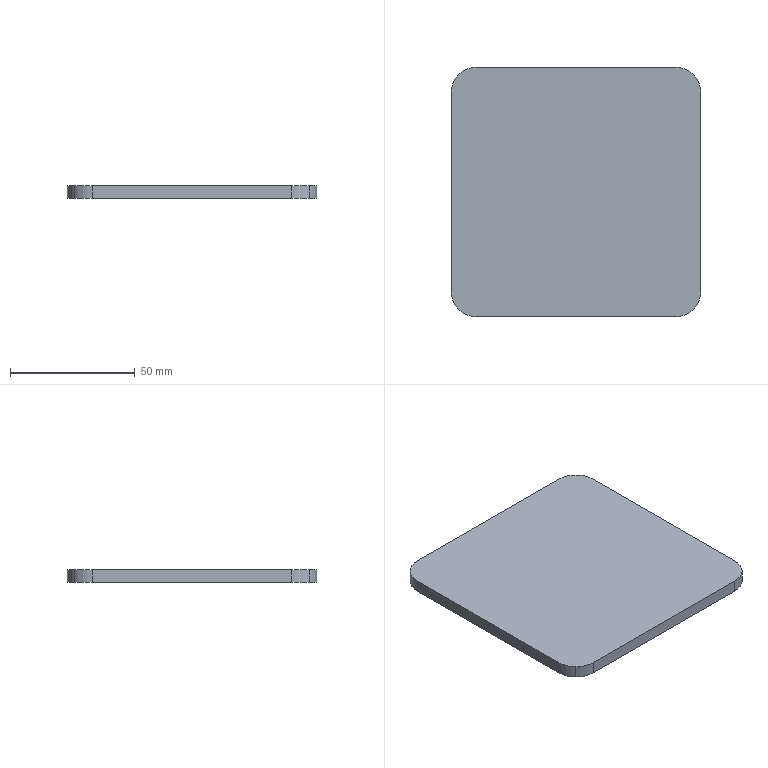Part | STEP file | DCV-000-024 | 1 solid | 14 faces | box 100 x 100 x 5 mm | volume 49571 mm3 | cylinder 8 | plane 6 | commonest cylinder face diameters 20 x8
STEP:
#1=CARTESIAN_POINT('',(0.,0.,0.));
#2=DIRECTION('',(0.,0.,1.));
#3=DIRECTION('',(1.,0.,0.));
#4=AXIS2_PLACEMENT_3D('',#1,#2,#3);
#5=CARTESIAN_POINT('',(40.,-50.,0.));
#6=VERTEX_POINT('',#5);
#7=CARTESIAN_POINT('',(47.071,-47.071,0.));
#8=VERTEX_POINT('',#7);
#9=CARTESIAN_POINT('',(40.,-40.,0.));
#10=DIRECTION('',(0.,0.,1.));
#11=DIRECTION('',(0.7071,-0.7071,0.));
#12=AXIS2_PLACEMENT_3D('',#9,#10,#11);
#13=CIRCLE('',#12,10.);
#14=CARTESIAN_POINT('',(40.,-40.,0.));
#15=DIRECTION('',(0.,0.,1.));
#16=DIRECTION('',(0.7071,-0.7071,0.));
#17=AXIS2_PLACEMENT_3D('',#14,#15,#16);
#18=CYLINDRICAL_SURFACE('',#17,10.);
#19=CARTESIAN_POINT('',(0.,0.));
#20=DIRECTION('',(1.,0.));
#21=VECTOR('',#20,1.);
#22=LINE('',#19,#21);
#23=(GEOMETRIC_REPRESENTATION_CONTEXT(2)PARAMETRIC_REPRESENTATION_CONTEXT()REPRESENTATION_CONTEXT('',''));
#24=DEFINITIONAL_REPRESENTATION('',(#22),#23);
#25=PCURVE('',#18,#24);
#26=CARTESIAN_POINT('',(0.,0.,0.));
#27=DIRECTION('',(0.,0.,1.));
#28=DIRECTION('',(1.,0.,0.));
#29=AXIS2_PLACEMENT_3D('',#26,#27,#28);
#30=PLANE('',#29);
#31=CARTESIAN_POINT('',(40.,-40.));
#32=DIRECTION('',(0.7071,-0.7071));
#33=AXIS2_PLACEMENT_2D('',#31,#32);
#34=CIRCLE('',#33,10.);
#35=(GEOMETRIC_REPRESENTATION_CONTEXT(2)PARAMETRIC_REPRESENTATION_CONTEXT()REPRESENTATION_CONTEXT('',''));
#36=DEFINITIONAL_REPRESENTATION('',(#34),#35);
#37=PCURVE('',#30,#36);
#38=SURFACE_CURVE('',#13,(#25,#37),.PCURVE_S1.);
#39=EDGE_CURVE('',#6,#8,#38,.T.);
#40=ORIENTED_EDGE('',*,*,#39,.T.);
#41=CARTESIAN_POINT('',(47.071,-47.071,5.));
#42=VERTEX_POINT('',#41);
#43=CARTESIAN_POINT('',(47.071,-47.071,0.));
#44=DIRECTION('',(0.,0.,1.));
#45=VECTOR('',#44,1.);
#46=LINE('',#43,#45);
#47=CARTESIAN_POINT('',(6.283,0.));
#48=DIRECTION('',(0.,1.));
#49=VECTOR('',#48,1.);
#50=LINE('',#47,#49);
#51=(GEOMETRIC_REPRESENTATION_CONTEXT(2)PARAMETRIC_REPRESENTATION_CONTEXT()REPRESENTATION_CONTEXT('',''));
#52=DEFINITIONAL_REPRESENTATION('',(#50),#51);
#53=PCURVE('',#18,#52);
#54=CARTESIAN_POINT('',(40.,-40.,0.));
#55=DIRECTION('',(0.,0.,1.));
#56=DIRECTION('',(0.7071,-0.7071,0.));
#57=AXIS2_PLACEMENT_3D('',#54,#55,#56);
#58=CYLINDRICAL_SURFACE('',#57,10.);
#59=CARTESIAN_POINT('',(0.,0.));
#60=DIRECTION('',(0.,1.));
#61=VECTOR('',#60,1.);
#62=LINE('',#59,#61);
#63=(GEOMETRIC_REPRESENTATION_CONTEXT(2)PARAMETRIC_REPRESENTATION_CONTEXT()REPRESENTATION_CONTEXT('',''));
#64=DEFINITIONAL_REPRESENTATION('',(#62),#63);
#65=PCURVE('',#58,#64);
#66=SURFACE_CURVE('',#46,(#53,#65),.PCURVE_S1.);
#67=EDGE_CURVE('',#8,#42,#66,.T.);
#68=ORIENTED_EDGE('',*,*,#67,.T.);
#69=CARTESIAN_POINT('',(40.,-50.,5.));
#70=VERTEX_POINT('',#69);
#71=CARTESIAN_POINT('',(40.,-40.,5.));
#72=DIRECTION('',(0.,0.,-1.));
#73=DIRECTION('',(0.7071,-0.7071,0.));
#74=AXIS2_PLACEMENT_3D('',#71,#72,#73);
#75=CIRCLE('',#74,10.);
#76=CARTESIAN_POINT('',(6.283,5.));
#77=DIRECTION('',(-1.,0.));
#78=VECTOR('',#77,1.);
#79=LINE('',#76,#78);
#80=(GEOMETRIC_REPRESENTATION_CONTEXT(2)PARAMETRIC_REPRESENTATION_CONTEXT()REPRESENTATION_CONTEXT('',''));
#81=DEFINITIONAL_REPRESENTATION('',(#79),#80);
#82=PCURVE('',#18,#81);
#83=CARTESIAN_POINT('',(0.,0.,5.));
#84=DIRECTION('',(0.,0.,1.));
#85=DIRECTION('',(1.,0.,0.));
#86=AXIS2_PLACEMENT_3D('',#83,#84,#85);
#87=PLANE('',#86);
#88=CARTESIAN_POINT('',(47.071,-47.071));
#89=CARTESIAN_POINT('',(34.824,-59.319));
#90=CARTESIAN_POINT('',(30.341,-42.588));
#91=CARTESIAN_POINT('',(25.858,-25.858));
#92=CARTESIAN_POINT('',(42.588,-30.341));
#93=CARTESIAN_POINT('',(59.319,-34.824));
#94=CARTESIAN_POINT('',(47.071,-47.071));
#95=(BOUNDED_CURVE()B_SPLINE_CURVE(2,(#88,#89,#90,#91,#92,#93,#94),.UNSPECIFIED.,.T.,.F.)B_SPLINE_CURVE_WITH_KNOTS((1,2,2,2,2,1),(-2.094,0.,2.094,4.189,6.283,8.378),.UNSPECIFIED.)CURVE()GEOMETRIC_REPRESENTATION_ITEM()RATIONAL_B_SPLINE_CURVE((1.,0.5,1.,0.5,1.,0.5,1.))REPRESENTATION_ITEM(''));
#96=(GEOMETRIC_REPRESENTATION_CONTEXT(2)PARAMETRIC_REPRESENTATION_CONTEXT()REPRESENTATION_CONTEXT('',''));
#97=DEFINITIONAL_REPRESENTATION('',(#95),#96);
#98=PCURVE('',#87,#97);
#99=SURFACE_CURVE('',#75,(#82,#98),.PCURVE_S1.);
#100=EDGE_CURVE('',#42,#70,#99,.T.);
#101=ORIENTED_EDGE('',*,*,#100,.T.);
#102=CARTESIAN_POINT('',(40.,-50.,0.));
#103=DIRECTION('',(0.,0.,-1.));
#104=VECTOR('',#103,1.);
#105=LINE('',#102,#104);
#106=CARTESIAN_POINT('',(5.498,0.));
#107=DIRECTION('',(0.,-1.));
#108=VECTOR('',#107,1.);
#109=LINE('',#106,#108);
#110=(GEOMETRIC_REPRESENTATION_CONTEXT(2)PARAMETRIC_REPRESENTATION_CONTEXT()REPRESENTATION_CONTEXT('',''));
#111=DEFINITIONAL_REPRESENTATION('',(#109),#110);
#112=PCURVE('',#18,#111);
#113=CARTESIAN_POINT('',(-50.,-50.,0.));
#114=DIRECTION('',(0.,-1.,0.));
#115=DIRECTION('',(0.,0.,-1.));
#116=AXIS2_PLACEMENT_3D('',#113,#114,#115);
#117=PLANE('',#116);
#118=CARTESIAN_POINT('',(0.,90.));
#119=DIRECTION('',(1.,0.));
#120=VECTOR('',#119,1.);
#121=LINE('',#118,#120);
#122=(GEOMETRIC_REPRESENTATION_CONTEXT(2)PARAMETRIC_REPRESENTATION_CONTEXT()REPRESENTATION_CONTEXT('',''));
#123=DEFINITIONAL_REPRESENTATION('',(#121),#122);
#124=PCURVE('',#117,#123);
#125=SURFACE_CURVE('',#105,(#112,#124),.PCURVE_S1.);
#126=EDGE_CURVE('',#70,#6,#125,.T.);
#127=ORIENTED_EDGE('',*,*,#126,.T.);
#128=EDGE_LOOP('',(#40,#68,#101,#127));
#129=FACE_BOUND('',#128,.T.);
#130=ADVANCED_FACE('',(#129),#18,.T.);
#131=CARTESIAN_POINT('',(-50.,-40.,0.));
#132=VERTEX_POINT('',#131);
#133=CARTESIAN_POINT('',(-47.071,-47.071,0.));
#134=VERTEX_POINT('',#133);
#135=CARTESIAN_POINT('',(-40.,-40.,0.));
#136=DIRECTION('',(0.,0.,1.));
#137=DIRECTION('',(-0.7071,-0.7071,0.));
#138=AXIS2_PLACEMENT_3D('',#135,#136,#137);
#139=CIRCLE('',#138,10.);
#140=CARTESIAN_POINT('',(-40.,-40.,0.));
#141=DIRECTION('',(0.,0.,1.));
#142=DIRECTION('',(-0.7071,-0.7071,0.));
#143=AXIS2_PLACEMENT_3D('',#140,#141,#142);
#144=CYLINDRICAL_SURFACE('',#143,10.);
#145=CARTESIAN_POINT('',(0.,0.));
#146=DIRECTION('',(1.,0.));
#147=VECTOR('',#146,1.);
#148=LINE('',#145,#147);
#149=(GEOMETRIC_REPRESENTATION_CONTEXT(2)PARAMETRIC_REPRESENTATION_CONTEXT()REPRESENTATION_CONTEXT('',''));
#150=DEFINITIONAL_REPRESENTATION('',(#148),#149);
#151=PCURVE('',#144,#150);
#152=CARTESIAN_POINT('',(-40.,-40.));
#153=DIRECTION('',(-0.7071,-0.7071));
#154=AXIS2_PLACEMENT_2D('',#152,#153);
#155=CIRCLE('',#154,10.);
#156=(GEOMETRIC_REPRESENTATION_CONTEXT(2)PARAMETRIC_REPRESENTATION_CONTEXT()REPRESENTATION_CONTEXT('',''));
#157=DEFINITIONAL_REPRESENTATION('',(#155),#156);
#158=PCURVE('',#30,#157);
#159=SURFACE_CURVE('',#139,(#151,#158),.PCURVE_S1.);
#160=EDGE_CURVE('',#132,#134,#159,.T.);
#161=ORIENTED_EDGE('',*,*,#160,.T.);
#162=CARTESIAN_POINT('',(-47.071,-47.071,5.));
#163=VERTEX_POINT('',#162);
#164=CARTESIAN_POINT('',(-47.071,-47.071,0.));
#165=DIRECTION('',(0.,0.,1.));
#166=VECTOR('',#165,1.);
#167=LINE('',#164,#166);
#168=CARTESIAN_POINT('',(6.283,0.));
#169=DIRECTION('',(0.,1.));
#170=VECTOR('',#169,1.);
#171=LINE('',#168,#170);
#172=(GEOMETRIC_REPRESENTATION_CONTEXT(2)PARAMETRIC_REPRESENTATION_CONTEXT()REPRESENTATION_CONTEXT('',''));
#173=DEFINITIONAL_REPRESENTATION('',(#171),#172);
#174=PCURVE('',#144,#173);
#175=CARTESIAN_POINT('',(-40.,-40.,0.));
#176=DIRECTION('',(0.,0.,1.));
#177=DIRECTION('',(-0.7071,-0.7071,0.));
#178=AXIS2_PLACEMENT_3D('',#175,#176,#177);
#179=CYLINDRICAL_SURFACE('',#178,10.);
#180=CARTESIAN_POINT('',(0.,0.));
#181=DIRECTION('',(0.,1.));
#182=VECTOR('',#181,1.);
#183=LINE('',#180,#182);
#184=(GEOMETRIC_REPRESENTATION_CONTEXT(2)PARAMETRIC_REPRESENTATION_CONTEXT()REPRESENTATION_CONTEXT('',''));
#185=DEFINITIONAL_REPRESENTATION('',(#183),#184);
#186=PCURVE('',#179,#185);
#187=SURFACE_CURVE('',#167,(#174,#186),.PCURVE_S1.);
#188=EDGE_CURVE('',#134,#163,#187,.T.);
#189=ORIENTED_EDGE('',*,*,#188,.T.);
#190=CARTESIAN_POINT('',(-50.,-40.,5.));
#191=VERTEX_POINT('',#190);
#192=CARTESIAN_POINT('',(-40.,-40.,5.));
#193=DIRECTION('',(0.,0.,-1.));
#194=DIRECTION('',(-0.7071,-0.7071,0.));
#195=AXIS2_PLACEMENT_3D('',#192,#193,#194);
#196=CIRCLE('',#195,10.);
#197=CARTESIAN_POINT('',(6.283,5.));
#198=DIRECTION('',(-1.,0.));
#199=VECTOR('',#198,1.);
#200=LINE('',#197,#199);
#201=(GEOMETRIC_REPRESENTATION_CONTEXT(2)PARAMETRIC_REPRESENTATION_CONTEXT()REPRESENTATION_CONTEXT('',''));
#202=DEFINITIONAL_REPRESENTATION('',(#200),#201);
#203=PCURVE('',#144,#202);
#204=CARTESIAN_POINT('',(-47.071,-47.071));
#205=CARTESIAN_POINT('',(-59.319,-34.824));
#206=CARTESIAN_POINT('',(-42.588,-30.341));
#207=CARTESIAN_POINT('',(-25.858,-25.858));
#208=CARTESIAN_POINT('',(-30.341,-42.588));
#209=CARTESIAN_POINT('',(-34.824,-59.319));
#210=CARTESIAN_POINT('',(-47.071,-47.071));
#211=(BOUNDED_CURVE()B_SPLINE_CURVE(2,(#204,#205,#206,#207,#208,#209,#210),.UNSPECIFIED.,.T.,.F.)B_SPLINE_CURVE_WITH_KNOTS((1,2,2,2,2,1),(-2.094,0.,2.094,4.189,6.283,8.378),.UNSPECIFIED.)CURVE()GEOMETRIC_REPRESENTATION_ITEM()RATIONAL_B_SPLINE_CURVE((1.,0.5,1.,0.5,1.,0.5,1.))REPRESENTATION_ITEM(''));
#212=(GEOMETRIC_REPRESENTATION_CONTEXT(2)PARAMETRIC_REPRESENTATION_CONTEXT()REPRESENTATION_CONTEXT('',''));
#213=DEFINITIONAL_REPRESENTATION('',(#211),#212);
#214=PCURVE('',#87,#213);
#215=SURFACE_CURVE('',#196,(#203,#214),.PCURVE_S1.);
#216=EDGE_CURVE('',#163,#191,#215,.T.);
#217=ORIENTED_EDGE('',*,*,#216,.T.);
#218=CARTESIAN_POINT('',(-50.,-40.,0.));
#219=DIRECTION('',(0.,0.,-1.));
#220=VECTOR('',#219,1.);
#221=LINE('',#218,#220);
#222=CARTESIAN_POINT('',(5.498,0.));
#223=DIRECTION('',(0.,-1.));
#224=VECTOR('',#223,1.);
#225=LINE('',#222,#224);
#226=(GEOMETRIC_REPRESENTATION_CONTEXT(2)PARAMETRIC_REPRESENTATION_CONTEXT()REPRESENTATION_CONTEXT('',''));
#227=DEFINITIONAL_REPRESENTATION('',(#225),#226);
#228=PCURVE('',#144,#227);
#229=CARTESIAN_POINT('',(-50.,50.,0.));
#230=DIRECTION('',(-1.,0.,0.));
#231=DIRECTION('',(0.,0.,1.));
#232=AXIS2_PLACEMENT_3D('',#229,#230,#231);
#233=PLANE('',#232);
#234=CARTESIAN_POINT('',(0.,-90.));
#235=DIRECTION('',(-1.,0.));
#236=VECTOR('',#235,1.);
#237=LINE('',#234,#236);
#238=(GEOMETRIC_REPRESENTATION_CONTEXT(2)PARAMETRIC_REPRESENTATION_CONTEXT()REPRESENTATION_CONTEXT('',''));
#239=DEFINITIONAL_REPRESENTATION('',(#237),#238);
#240=PCURVE('',#233,#239);
#241=SURFACE_CURVE('',#221,(#228,#240),.PCURVE_S1.);
#242=EDGE_CURVE('',#191,#132,#241,.T.);
#243=ORIENTED_EDGE('',*,*,#242,.T.);
#244=EDGE_LOOP('',(#161,#189,#217,#243));
#245=FACE_BOUND('',#244,.T.);
#246=ADVANCED_FACE('',(#245),#144,.T.);
#247=CARTESIAN_POINT('',(-40.,50.,0.));
#248=VERTEX_POINT('',#247);
#249=CARTESIAN_POINT('',(-47.071,47.071,0.));
#250=VERTEX_POINT('',#249);
#251=CARTESIAN_POINT('',(-40.,40.,0.));
#252=DIRECTION('',(0.,0.,1.));
#253=DIRECTION('',(-0.7071,0.7071,0.));
#254=AXIS2_PLACEMENT_3D('',#251,#252,#253);
#255=CIRCLE('',#254,10.);
#256=CARTESIAN_POINT('',(-40.,40.,0.));
#257=DIRECTION('',(0.,0.,1.));
#258=DIRECTION('',(-0.7071,0.7071,0.));
#259=AXIS2_PLACEMENT_3D('',#256,#257,#258);
#260=CYLINDRICAL_SURFACE('',#259,10.);
#261=CARTESIAN_POINT('',(0.,0.));
#262=DIRECTION('',(1.,0.));
#263=VECTOR('',#262,1.);
#264=LINE('',#261,#263);
#265=(GEOMETRIC_REPRESENTATION_CONTEXT(2)PARAMETRIC_REPRESENTATION_CONTEXT()REPRESENTATION_CONTEXT('',''));
#266=DEFINITIONAL_REPRESENTATION('',(#264),#265);
#267=PCURVE('',#260,#266);
#268=CARTESIAN_POINT('',(-40.,40.));
#269=DIRECTION('',(-0.7071,0.7071));
#270=AXIS2_PLACEMENT_2D('',#268,#269);
#271=CIRCLE('',#270,10.);
#272=(GEOMETRIC_REPRESENTATION_CONTEXT(2)PARAMETRIC_REPRESENTATION_CONTEXT()REPRESENTATION_CONTEXT('',''));
#273=DEFINITIONAL_REPRESENTATION('',(#271),#272);
#274=PCURVE('',#30,#273);
#275=SURFACE_CURVE('',#255,(#267,#274),.PCURVE_S1.);
#276=EDGE_CURVE('',#248,#250,#275,.T.);
#277=ORIENTED_EDGE('',*,*,#276,.T.);
#278=CARTESIAN_POINT('',(-47.071,47.071,5.));
#279=VERTEX_POINT('',#278);
#280=CARTESIAN_POINT('',(-47.071,47.071,0.));
#281=DIRECTION('',(0.,0.,1.));
#282=VECTOR('',#281,1.);
#283=LINE('',#280,#282);
#284=CARTESIAN_POINT('',(6.283,0.));
#285=DIRECTION('',(0.,1.));
#286=VECTOR('',#285,1.);
#287=LINE('',#284,#286);
#288=(GEOMETRIC_REPRESENTATION_CONTEXT(2)PARAMETRIC_REPRESENTATION_CONTEXT()REPRESENTATION_CONTEXT('',''));
#289=DEFINITIONAL_REPRESENTATION('',(#287),#288);
#290=PCURVE('',#260,#289);
#291=CARTESIAN_POINT('',(-40.,40.,0.));
#292=DIRECTION('',(0.,0.,1.));
#293=DIRECTION('',(-0.7071,0.7071,0.));
#294=AXIS2_PLACEMENT_3D('',#291,#292,#293);
#295=CYLINDRICAL_SURFACE('',#294,10.);
#296=CARTESIAN_POINT('',(0.,0.));
#297=DIRECTION('',(0.,1.));
#298=VECTOR('',#297,1.);
#299=LINE('',#296,#298);
#300=(GEOMETRIC_REPRESENTATION_CONTEXT(2)PARAMETRIC_REPRESENTATION_CONTEXT()REPRESENTATION_CONTEXT('',''));
#301=DEFINITIONAL_REPRESENTATION('',(#299),#300);
#302=PCURVE('',#295,#301);
#303=SURFACE_CURVE('',#283,(#290,#302),.PCURVE_S1.);
#304=EDGE_CURVE('',#250,#279,#303,.T.);
#305=ORIENTED_EDGE('',*,*,#304,.T.);
#306=CARTESIAN_POINT('',(-40.,50.,5.));
#307=VERTEX_POINT('',#306);
#308=CARTESIAN_POINT('',(-40.,40.,5.));
#309=DIRECTION('',(0.,0.,-1.));
#310=DIRECTION('',(-0.7071,0.7071,0.));
#311=AXIS2_PLACEMENT_3D('',#308,#309,#310);
#312=CIRCLE('',#311,10.);
#313=CARTESIAN_POINT('',(6.283,5.));
#314=DIRECTION('',(-1.,0.));
#315=VECTOR('',#314,1.);
#316=LINE('',#313,#315);
#317=(GEOMETRIC_REPRESENTATION_CONTEXT(2)PARAMETRIC_REPRESENTATION_CONTEXT()REPRESENTATION_CONTEXT('',''));
#318=DEFINITIONAL_REPRESENTATION('',(#316),#317);
#319=PCURVE('',#260,#318);
#320=CARTESIAN_POINT('',(-47.071,47.071));
#321=CARTESIAN_POINT('',(-34.824,59.319));
#322=CARTESIAN_POINT('',(-30.341,42.588));
#323=CARTESIAN_POINT('',(-25.858,25.858));
#324=CARTESIAN_POINT('',(-42.588,30.341));
#325=CARTESIAN_POINT('',(-59.319,34.824));
#326=CARTESIAN_POINT('',(-47.071,47.071));
#327=(BOUNDED_CURVE()B_SPLINE_CURVE(2,(#320,#321,#322,#323,#324,#325,#326),.UNSPECIFIED.,.T.,.F.)B_SPLINE_CURVE_WITH_KNOTS((1,2,2,2,2,1),(-2.094,0.,2.094,4.189,6.283,8.378),.UNSPECIFIED.)CURVE()GEOMETRIC_REPRESENTATION_ITEM()RATIONAL_B_SPLINE_CURVE((1.,0.5,1.,0.5,1.,0.5,1.))REPRESENTATION_ITEM(''));
#328=(GEOMETRIC_REPRESENTATION_CONTEXT(2)PARAMETRIC_REPRESENTATION_CONTEXT()REPRESENTATION_CONTEXT('',''));
#329=DEFINITIONAL_REPRESENTATION('',(#327),#328);
#330=PCURVE('',#87,#329);
#331=SURFACE_CURVE('',#312,(#319,#330),.PCURVE_S1.);
#332=EDGE_CURVE('',#279,#307,#331,.T.);
#333=ORIENTED_EDGE('',*,*,#332,.T.);
#334=CARTESIAN_POINT('',(-40.,50.,0.));
#335=DIRECTION('',(0.,0.,-1.));
#336=VECTOR('',#335,1.);
#337=LINE('',#334,#336);
#338=CARTESIAN_POINT('',(5.498,0.));
#339=DIRECTION('',(0.,-1.));
#340=VECTOR('',#339,1.);
#341=LINE('',#338,#340);
#342=(GEOMETRIC_REPRESENTATION_CONTEXT(2)PARAMETRIC_REPRESENTATION_CONTEXT()REPRESENTATION_CONTEXT('',''));
#343=DEFINITIONAL_REPRESENTATION('',(#341),#342);
#344=PCURVE('',#260,#343);
#345=CARTESIAN_POINT('',(50.,50.,0.));
#346=DIRECTION('',(0.,1.,0.));
#347=DIRECTION('',(1.,0.,0.));
#348=AXIS2_PLACEMENT_3D('',#345,#346,#347);
#349=PLANE('',#348);
#350=CARTESIAN_POINT('',(-90.,0.));
#351=DIRECTION('',(0.,1.));
#352=VECTOR('',#351,1.);
#353=LINE('',#350,#352);
#354=(GEOMETRIC_REPRESENTATION_CONTEXT(2)PARAMETRIC_REPRESENTATION_CONTEXT()REPRESENTATION_CONTEXT('',''));
#355=DEFINITIONAL_REPRESENTATION('',(#353),#354);
#356=PCURVE('',#349,#355);
#357=SURFACE_CURVE('',#337,(#344,#356),.PCURVE_S1.);
#358=EDGE_CURVE('',#307,#248,#357,.T.);
#359=ORIENTED_EDGE('',*,*,#358,.T.);
#360=EDGE_LOOP('',(#277,#305,#333,#359));
#361=FACE_BOUND('',#360,.T.);
#362=ADVANCED_FACE('',(#361),#260,.T.);
#363=CARTESIAN_POINT('',(50.,40.,0.));
#364=VERTEX_POINT('',#363);
#365=CARTESIAN_POINT('',(47.071,47.071,0.));
#366=VERTEX_POINT('',#365);
#367=CARTESIAN_POINT('',(40.,40.,0.));
#368=DIRECTION('',(0.,0.,1.));
#369=DIRECTION('',(0.7071,0.7071,0.));
#370=AXIS2_PLACEMENT_3D('',#367,#368,#369);
#371=CIRCLE('',#370,10.);
#372=CARTESIAN_POINT('',(40.,40.,0.));
#373=DIRECTION('',(0.,0.,1.));
#374=DIRECTION('',(0.7071,0.7071,0.));
#375=AXIS2_PLACEMENT_3D('',#372,#373,#374);
#376=CYLINDRICAL_SURFACE('',#375,10.);
#377=CARTESIAN_POINT('',(0.,0.));
#378=DIRECTION('',(1.,0.));
#379=VECTOR('',#378,1.);
#380=LINE('',#377,#379);
#381=(GEOMETRIC_REPRESENTATION_CONTEXT(2)PARAMETRIC_REPRESENTATION_CONTEXT()REPRESENTATION_CONTEXT('',''));
#382=DEFINITIONAL_REPRESENTATION('',(#380),#381);
#383=PCURVE('',#376,#382);
#384=CARTESIAN_POINT('',(40.,40.));
#385=DIRECTION('',(0.7071,0.7071));
#386=AXIS2_PLACEMENT_2D('',#384,#385);
#387=CIRCLE('',#386,10.);
#388=(GEOMETRIC_REPRESENTATION_CONTEXT(2)PARAMETRIC_REPRESENTATION_CONTEXT()REPRESENTATION_CONTEXT('',''));
#389=DEFINITIONAL_REPRESENTATION('',(#387),#388);
#390=PCURVE('',#30,#389);
#391=SURFACE_CURVE('',#371,(#383,#390),.PCURVE_S1.);
#392=EDGE_CURVE('',#364,#366,#391,.T.);
#393=ORIENTED_EDGE('',*,*,#392,.T.);
#394=CARTESIAN_POINT('',(47.071,47.071,5.));
#395=VERTEX_POINT('',#394);
#396=CARTESIAN_POINT('',(47.071,47.071,0.));
#397=DIRECTION('',(0.,0.,1.));
#398=VECTOR('',#397,1.);
#399=LINE('',#396,#398);
#400=CARTESIAN_POINT('',(6.283,0.));
#401=DIRECTION('',(0.,1.));
#402=VECTOR('',#401,1.);
#403=LINE('',#400,#402);
#404=(GEOMETRIC_REPRESENTATION_CONTEXT(2)PARAMETRIC_REPRESENTATION_CONTEXT()REPRESENTATION_CONTEXT('',''));
#405=DEFINITIONAL_REPRESENTATION('',(#403),#404);
#406=PCURVE('',#376,#405);
#407=CARTESIAN_POINT('',(40.,40.,0.));
#408=DIRECTION('',(0.,0.,1.));
#409=DIRECTION('',(0.7071,0.7071,0.));
#410=AXIS2_PLACEMENT_3D('',#407,#408,#409);
#411=CYLINDRICAL_SURFACE('',#410,10.);
#412=CARTESIAN_POINT('',(0.,0.));
#413=DIRECTION('',(0.,1.));
#414=VECTOR('',#413,1.);
#415=LINE('',#412,#414);
#416=(GEOMETRIC_REPRESENTATION_CONTEXT(2)PARAMETRIC_REPRESENTATION_CONTEXT()REPRESENTATION_CONTEXT('',''));
#417=DEFINITIONAL_REPRESENTATION('',(#415),#416);
#418=PCURVE('',#411,#417);
#419=SURFACE_CURVE('',#399,(#406,#418),.PCURVE_S1.);
#420=EDGE_CURVE('',#366,#395,#419,.T.);
#421=ORIENTED_EDGE('',*,*,#420,.T.);
#422=CARTESIAN_POINT('',(50.,40.,5.));
#423=VERTEX_POINT('',#422);
#424=CARTESIAN_POINT('',(40.,40.,5.));
#425=DIRECTION('',(0.,0.,-1.));
#426=DIRECTION('',(0.7071,0.7071,0.));
#427=AXIS2_PLACEMENT_3D('',#424,#425,#426);
#428=CIRCLE('',#427,10.);
#429=CARTESIAN_POINT('',(6.283,5.));
#430=DIRECTION('',(-1.,0.));
#431=VECTOR('',#430,1.);
#432=LINE('',#429,#431);
#433=(GEOMETRIC_REPRESENTATION_CONTEXT(2)PARAMETRIC_REPRESENTATION_CONTEXT()REPRESENTATION_CONTEXT('',''));
#434=DEFINITIONAL_REPRESENTATION('',(#432),#433);
#435=PCURVE('',#376,#434);
#436=CARTESIAN_POINT('',(47.071,47.071));
#437=CARTESIAN_POINT('',(59.319,34.824));
#438=CARTESIAN_POINT('',(42.588,30.341));
#439=CARTESIAN_POINT('',(25.858,25.858));
#440=CARTESIAN_POINT('',(30.341,42.588));
#441=CARTESIAN_POINT('',(34.824,59.319));
#442=CARTESIAN_POINT('',(47.071,47.071));
#443=(BOUNDED_CURVE()B_SPLINE_CURVE(2,(#436,#437,#438,#439,#440,#441,#442),.UNSPECIFIED.,.T.,.F.)B_SPLINE_CURVE_WITH_KNOTS((1,2,2,2,2,1),(-2.094,0.,2.094,4.189,6.283,8.378),.UNSPECIFIED.)CURVE()GEOMETRIC_REPRESENTATION_ITEM()RATIONAL_B_SPLINE_CURVE((1.,0.5,1.,0.5,1.,0.5,1.))REPRESENTATION_ITEM(''));
#444=(GEOMETRIC_REPRESENTATION_CONTEXT(2)PARAMETRIC_REPRESENTATION_CONTEXT()REPRESENTATION_CONTEXT('',''));
#445=DEFINITIONAL_REPRESENTATION('',(#443),#444);
#446=PCURVE('',#87,#445);
#447=SURFACE_CURVE('',#428,(#435,#446),.PCURVE_S1.);
#448=EDGE_CURVE('',#395,#423,#447,.T.);
#449=ORIENTED_EDGE('',*,*,#448,.T.);
#450=CARTESIAN_POINT('',(50.,40.,0.));
#451=DIRECTION('',(0.,0.,-1.));
#452=VECTOR('',#451,1.);
#453=LINE('',#450,#452);
#454=CARTESIAN_POINT('',(5.498,0.));
#455=DIRECTION('',(0.,-1.));
#456=VECTOR('',#455,1.);
#457=LINE('',#454,#456);
#458=(GEOMETRIC_REPRESENTATION_CONTEXT(2)PARAMETRIC_REPRESENTATION_CONTEXT()REPRESENTATION_CONTEXT('',''));
#459=DEFINITIONAL_REPRESENTATION('',(#457),#458);
#460=PCURVE('',#376,#459);
#461=CARTESIAN_POINT('',(50.,-50.,0.));
#462=DIRECTION('',(1.,0.,0.));
#463=DIRECTION('',(0.,1.,0.));
#464=AXIS2_PLACEMENT_3D('',#461,#462,#463);
#465=PLANE('',#464);
#466=CARTESIAN_POINT('',(90.,0.));
#467=DIRECTION('',(0.,-1.));
#468=VECTOR('',#467,1.);
#469=LINE('',#466,#468);
#470=(GEOMETRIC_REPRESENTATION_CONTEXT(2)PARAMETRIC_REPRESENTATION_CONTEXT()REPRESENTATION_CONTEXT('',''));
#471=DEFINITIONAL_REPRESENTATION('',(#469),#470);
#472=PCURVE('',#465,#471);
#473=SURFACE_CURVE('',#453,(#460,#472),.PCURVE_S1.);
#474=EDGE_CURVE('',#423,#364,#473,.T.);
#475=ORIENTED_EDGE('',*,*,#474,.T.);
#476=EDGE_LOOP('',(#393,#421,#449,#475));
#477=FACE_BOUND('',#476,.T.);
#478=ADVANCED_FACE('',(#477),#376,.T.);
#479=CARTESIAN_POINT('',(50.,-40.,5.));
#480=VERTEX_POINT('',#479);
#481=CARTESIAN_POINT('',(40.,-40.,5.));
#482=DIRECTION('',(0.,0.,-1.));
#483=DIRECTION('',(0.7071,-0.7071,0.));
#484=AXIS2_PLACEMENT_3D('',#481,#482,#483);
#485=CIRCLE('',#484,10.);
#486=CARTESIAN_POINT('',(47.071,-47.071));
#487=CARTESIAN_POINT('',(34.824,-59.319));
#488=CARTESIAN_POINT('',(30.341,-42.588));
#489=CARTESIAN_POINT('',(25.858,-25.858));
#490=CARTESIAN_POINT('',(42.588,-30.341));
#491=CARTESIAN_POINT('',(59.319,-34.824));
#492=CARTESIAN_POINT('',(47.071,-47.071));
#493=(BOUNDED_CURVE()B_SPLINE_CURVE(2,(#486,#487,#488,#489,#490,#491,#492),.UNSPECIFIED.,.T.,.F.)B_SPLINE_CURVE_WITH_KNOTS((1,2,2,2,2,1),(-2.094,0.,2.094,4.189,6.283,8.378),.UNSPECIFIED.)CURVE()GEOMETRIC_REPRESENTATION_ITEM()RATIONAL_B_SPLINE_CURVE((1.,0.5,1.,0.5,1.,0.5,1.))REPRESENTATION_ITEM(''));
#494=(GEOMETRIC_REPRESENTATION_CONTEXT(2)PARAMETRIC_REPRESENTATION_CONTEXT()REPRESENTATION_CONTEXT('',''));
#495=DEFINITIONAL_REPRESENTATION('',(#493),#494);
#496=PCURVE('',#87,#495);
#497=CARTESIAN_POINT('',(6.283,5.));
#498=DIRECTION('',(-1.,0.));
#499=VECTOR('',#498,1.);
#500=LINE('',#497,#499);
#501=(GEOMETRIC_REPRESENTATION_CONTEXT(2)PARAMETRIC_REPRESENTATION_CONTEXT()REPRESENTATION_CONTEXT('',''));
#502=DEFINITIONAL_REPRESENTATION('',(#500),#501);
#503=PCURVE('',#58,#502);
#504=SURFACE_CURVE('',#485,(#496,#503),.PCURVE_S1.);
#505=EDGE_CURVE('',#480,#42,#504,.T.);
#506=ORIENTED_EDGE('',*,*,#505,.F.);
#507=CARTESIAN_POINT('',(50.,-50.,5.));
#508=DIRECTION('',(0.,1.,0.));
#509=VECTOR('',#508,1.);
#510=LINE('',#507,#509);
#511=CARTESIAN_POINT('',(50.,-50.));
#512=DIRECTION('',(0.,1.));
#513=VECTOR('',#512,1.);
#514=LINE('',#511,#513);
#515=(GEOMETRIC_REPRESENTATION_CONTEXT(2)PARAMETRIC_REPRESENTATION_CONTEXT()REPRESENTATION_CONTEXT('',''));
#516=DEFINITIONAL_REPRESENTATION('',(#514),#515);
#517=PCURVE('',#87,#516);
#518=CARTESIAN_POINT('',(0.,5.));
#519=DIRECTION('',(1.,0.));
#520=VECTOR('',#519,1.);
#521=LINE('',#518,#520);
#522=(GEOMETRIC_REPRESENTATION_CONTEXT(2)PARAMETRIC_REPRESENTATION_CONTEXT()REPRESENTATION_CONTEXT('',''));
#523=DEFINITIONAL_REPRESENTATION('',(#521),#522);
#524=PCURVE('',#465,#523);
#525=SURFACE_CURVE('',#510,(#517,#524),.PCURVE_S1.);
#526=EDGE_CURVE('',#480,#423,#525,.T.);
#527=ORIENTED_EDGE('',*,*,#526,.T.);
#528=ORIENTED_EDGE('',*,*,#448,.F.);
#529=CARTESIAN_POINT('',(40.,50.,5.));
#530=VERTEX_POINT('',#529);
#531=CARTESIAN_POINT('',(40.,40.,5.));
#532=DIRECTION('',(0.,0.,-1.));
#533=DIRECTION('',(0.7071,0.7071,0.));
#534=AXIS2_PLACEMENT_3D('',#531,#532,#533);
#535=CIRCLE('',#534,10.);
#536=CARTESIAN_POINT('',(47.071,47.071));
#537=CARTESIAN_POINT('',(59.319,34.824));
#538=CARTESIAN_POINT('',(42.588,30.341));
#539=CARTESIAN_POINT('',(25.858,25.858));
#540=CARTESIAN_POINT('',(30.341,42.588));
#541=CARTESIAN_POINT('',(34.824,59.319));
#542=CARTESIAN_POINT('',(47.071,47.071));
#543=(BOUNDED_CURVE()B_SPLINE_CURVE(2,(#536,#537,#538,#539,#540,#541,#542),.UNSPECIFIED.,.T.,.F.)B_SPLINE_CURVE_WITH_KNOTS((1,2,2,2,2,1),(-2.094,0.,2.094,4.189,6.283,8.378),.UNSPECIFIED.)CURVE()GEOMETRIC_REPRESENTATION_ITEM()RATIONAL_B_SPLINE_CURVE((1.,0.5,1.,0.5,1.,0.5,1.))REPRESENTATION_ITEM(''));
#544=(GEOMETRIC_REPRESENTATION_CONTEXT(2)PARAMETRIC_REPRESENTATION_CONTEXT()REPRESENTATION_CONTEXT('',''));
#545=DEFINITIONAL_REPRESENTATION('',(#543),#544);
#546=PCURVE('',#87,#545);
#547=CARTESIAN_POINT('',(6.283,5.));
#548=DIRECTION('',(-1.,0.));
#549=VECTOR('',#548,1.);
#550=LINE('',#547,#549);
#551=(GEOMETRIC_REPRESENTATION_CONTEXT(2)PARAMETRIC_REPRESENTATION_CONTEXT()REPRESENTATION_CONTEXT('',''));
#552=DEFINITIONAL_REPRESENTATION('',(#550),#551);
#553=PCURVE('',#411,#552);
#554=SURFACE_CURVE('',#535,(#546,#553),.PCURVE_S1.);
#555=EDGE_CURVE('',#530,#395,#554,.T.);
#556=ORIENTED_EDGE('',*,*,#555,.F.);
#557=CARTESIAN_POINT('',(50.,50.,5.));
#558=DIRECTION('',(-1.,0.,0.));
#559=VECTOR('',#558,1.);
#560=LINE('',#557,#559);
#561=CARTESIAN_POINT('',(50.,50.));
#562=DIRECTION('',(-1.,0.));
#563=VECTOR('',#562,1.);
#564=LINE('',#561,#563);
#565=(GEOMETRIC_REPRESENTATION_CONTEXT(2)PARAMETRIC_REPRESENTATION_CONTEXT()REPRESENTATION_CONTEXT('',''));
#566=DEFINITIONAL_REPRESENTATION('',(#564),#565);
#567=PCURVE('',#87,#566);
#568=CARTESIAN_POINT('',(0.,-5.));
#569=DIRECTION('',(-1.,0.));
#570=VECTOR('',#569,1.);
#571=LINE('',#568,#570);
#572=(GEOMETRIC_REPRESENTATION_CONTEXT(2)PARAMETRIC_REPRESENTATION_CONTEXT()REPRESENTATION_CONTEXT('',''));
#573=DEFINITIONAL_REPRESENTATION('',(#571),#572);
#574=PCURVE('',#349,#573);
#575=SURFACE_CURVE('',#560,(#567,#574),.PCURVE_S1.);
#576=EDGE_CURVE('',#530,#307,#575,.T.);
#577=ORIENTED_EDGE('',*,*,#576,.T.);
#578=ORIENTED_EDGE('',*,*,#332,.F.);
#579=CARTESIAN_POINT('',(-50.,40.,5.));
#580=VERTEX_POINT('',#579);
#581=CARTESIAN_POINT('',(-40.,40.,5.));
#582=DIRECTION('',(0.,0.,-1.));
#583=DIRECTION('',(-0.7071,0.7071,0.));
#584=AXIS2_PLACEMENT_3D('',#581,#582,#583);
#585=CIRCLE('',#584,10.);
#586=CARTESIAN_POINT('',(-47.071,47.071));
#587=CARTESIAN_POINT('',(-34.824,59.319));
#588=CARTESIAN_POINT('',(-30.341,42.588));
#589=CARTESIAN_POINT('',(-25.858,25.858));
#590=CARTESIAN_POINT('',(-42.588,30.341));
#591=CARTESIAN_POINT('',(-59.319,34.824));
#592=CARTESIAN_POINT('',(-47.071,47.071));
#593=(BOUNDED_CURVE()B_SPLINE_CURVE(2,(#586,#587,#588,#589,#590,#591,#592),.UNSPECIFIED.,.T.,.F.)B_SPLINE_CURVE_WITH_KNOTS((1,2,2,2,2,1),(-2.094,0.,2.094,4.189,6.283,8.378),.UNSPECIFIED.)CURVE()GEOMETRIC_REPRESENTATION_ITEM()RATIONAL_B_SPLINE_CURVE((1.,0.5,1.,0.5,1.,0.5,1.))REPRESENTATION_ITEM(''));
#594=(GEOMETRIC_REPRESENTATION_CONTEXT(2)PARAMETRIC_REPRESENTATION_CONTEXT()REPRESENTATION_CONTEXT('',''));
#595=DEFINITIONAL_REPRESENTATION('',(#593),#594);
#596=PCURVE('',#87,#595);
#597=CARTESIAN_POINT('',(6.283,5.));
#598=DIRECTION('',(-1.,0.));
#599=VECTOR('',#598,1.);
#600=LINE('',#597,#599);
#601=(GEOMETRIC_REPRESENTATION_CONTEXT(2)PARAMETRIC_REPRESENTATION_CONTEXT()REPRESENTATION_CONTEXT('',''));
#602=DEFINITIONAL_REPRESENTATION('',(#600),#601);
#603=PCURVE('',#295,#602);
#604=SURFACE_CURVE('',#585,(#596,#603),.PCURVE_S1.);
#605=EDGE_CURVE('',#580,#279,#604,.T.);
#606=ORIENTED_EDGE('',*,*,#605,.F.);
#607=CARTESIAN_POINT('',(-50.,50.,5.));
#608=DIRECTION('',(0.,-1.,0.));
#609=VECTOR('',#608,1.);
#610=LINE('',#607,#609);
#611=CARTESIAN_POINT('',(-50.,50.));
#612=DIRECTION('',(0.,-1.));
#613=VECTOR('',#612,1.);
#614=LINE('',#611,#613);
#615=(GEOMETRIC_REPRESENTATION_CONTEXT(2)PARAMETRIC_REPRESENTATION_CONTEXT()REPRESENTATION_CONTEXT('',''));
#616=DEFINITIONAL_REPRESENTATION('',(#614),#615);
#617=PCURVE('',#87,#616);
#618=CARTESIAN_POINT('',(5.,0.));
#619=DIRECTION('',(0.,-1.));
#620=VECTOR('',#619,1.);
#621=LINE('',#618,#620);
#622=(GEOMETRIC_REPRESENTATION_CONTEXT(2)PARAMETRIC_REPRESENTATION_CONTEXT()REPRESENTATION_CONTEXT('',''));
#623=DEFINITIONAL_REPRESENTATION('',(#621),#622);
#624=PCURVE('',#233,#623);
#625=SURFACE_CURVE('',#610,(#617,#624),.PCURVE_S1.);
#626=EDGE_CURVE('',#580,#191,#625,.T.);
#627=ORIENTED_EDGE('',*,*,#626,.T.);
#628=ORIENTED_EDGE('',*,*,#216,.F.);
#629=CARTESIAN_POINT('',(-40.,-50.,5.));
#630=VERTEX_POINT('',#629);
#631=CARTESIAN_POINT('',(-40.,-40.,5.));
#632=DIRECTION('',(0.,0.,-1.));
#633=DIRECTION('',(-0.7071,-0.7071,0.));
#634=AXIS2_PLACEMENT_3D('',#631,#632,#633);
#635=CIRCLE('',#634,10.);
#636=CARTESIAN_POINT('',(-47.071,-47.071));
#637=CARTESIAN_POINT('',(-59.319,-34.824));
#638=CARTESIAN_POINT('',(-42.588,-30.341));
#639=CARTESIAN_POINT('',(-25.858,-25.858));
#640=CARTESIAN_POINT('',(-30.341,-42.588));
#641=CARTESIAN_POINT('',(-34.824,-59.319));
#642=CARTESIAN_POINT('',(-47.071,-47.071));
#643=(BOUNDED_CURVE()B_SPLINE_CURVE(2,(#636,#637,#638,#639,#640,#641,#642),.UNSPECIFIED.,.T.,.F.)B_SPLINE_CURVE_WITH_KNOTS((1,2,2,2,2,1),(-2.094,0.,2.094,4.189,6.283,8.378),.UNSPECIFIED.)CURVE()GEOMETRIC_REPRESENTATION_ITEM()RATIONAL_B_SPLINE_CURVE((1.,0.5,1.,0.5,1.,0.5,1.))REPRESENTATION_ITEM(''));
#644=(GEOMETRIC_REPRESENTATION_CONTEXT(2)PARAMETRIC_REPRESENTATION_CONTEXT()REPRESENTATION_CONTEXT('',''));
#645=DEFINITIONAL_REPRESENTATION('',(#643),#644);
#646=PCURVE('',#87,#645);
#647=CARTESIAN_POINT('',(6.283,5.));
#648=DIRECTION('',(-1.,0.));
#649=VECTOR('',#648,1.);
#650=LINE('',#647,#649);
#651=(GEOMETRIC_REPRESENTATION_CONTEXT(2)PARAMETRIC_REPRESENTATION_CONTEXT()REPRESENTATION_CONTEXT('',''));
#652=DEFINITIONAL_REPRESENTATION('',(#650),#651);
#653=PCURVE('',#179,#652);
#654=SURFACE_CURVE('',#635,(#646,#653),.PCURVE_S1.);
#655=EDGE_CURVE('',#630,#163,#654,.T.);
#656=ORIENTED_EDGE('',*,*,#655,.F.);
#657=CARTESIAN_POINT('',(-50.,-50.,5.));
#658=DIRECTION('',(1.,0.,0.));
#659=VECTOR('',#658,1.);
#660=LINE('',#657,#659);
#661=CARTESIAN_POINT('',(-50.,-50.));
#662=DIRECTION('',(1.,0.));
#663=VECTOR('',#662,1.);
#664=LINE('',#661,#663);
#665=(GEOMETRIC_REPRESENTATION_CONTEXT(2)PARAMETRIC_REPRESENTATION_CONTEXT()REPRESENTATION_CONTEXT('',''));
#666=DEFINITIONAL_REPRESENTATION('',(#664),#665);
#667=PCURVE('',#87,#666);
#668=CARTESIAN_POINT('',(-5.,0.));
#669=DIRECTION('',(0.,1.));
#670=VECTOR('',#669,1.);
#671=LINE('',#668,#670);
#672=(GEOMETRIC_REPRESENTATION_CONTEXT(2)PARAMETRIC_REPRESENTATION_CONTEXT()REPRESENTATION_CONTEXT('',''));
#673=DEFINITIONAL_REPRESENTATION('',(#671),#672);
#674=PCURVE('',#117,#673);
#675=SURFACE_CURVE('',#660,(#667,#674),.PCURVE_S1.);
#676=EDGE_CURVE('',#630,#70,#675,.T.);
#677=ORIENTED_EDGE('',*,*,#676,.T.);
#678=ORIENTED_EDGE('',*,*,#100,.F.);
#679=EDGE_LOOP('',(#506,#527,#528,#556,#577,#578,#606,#627,#628,#656,#677,#678));
#680=FACE_BOUND('',#679,.T.);
#681=ADVANCED_FACE('',(#680),#87,.T.);
#682=ORIENTED_EDGE('',*,*,#358,.F.);
#683=ORIENTED_EDGE('',*,*,#576,.F.);
#684=CARTESIAN_POINT('',(40.,50.,0.));
#685=VERTEX_POINT('',#684);
#686=CARTESIAN_POINT('',(40.,50.,0.));
#687=DIRECTION('',(0.,0.,1.));
#688=VECTOR('',#687,1.);
#689=LINE('',#686,#688);
#690=CARTESIAN_POINT('',(-10.,0.));
#691=DIRECTION('',(0.,-1.));
#692=VECTOR('',#691,1.);
#693=LINE('',#690,#692);
#694=(GEOMETRIC_REPRESENTATION_CONTEXT(2)PARAMETRIC_REPRESENTATION_CONTEXT()REPRESENTATION_CONTEXT('',''));
#695=DEFINITIONAL_REPRESENTATION('',(#693),#694);
#696=PCURVE('',#349,#695);
#697=CARTESIAN_POINT('',(0.7854,0.));
#698=DIRECTION('',(0.,1.));
#699=VECTOR('',#698,1.);
#700=LINE('',#697,#699);
#701=(GEOMETRIC_REPRESENTATION_CONTEXT(2)PARAMETRIC_REPRESENTATION_CONTEXT()REPRESENTATION_CONTEXT('',''));
#702=DEFINITIONAL_REPRESENTATION('',(#700),#701);
#703=PCURVE('',#411,#702);
#704=SURFACE_CURVE('',#689,(#696,#703),.PCURVE_S1.);
#705=EDGE_CURVE('',#685,#530,#704,.T.);
#706=ORIENTED_EDGE('',*,*,#705,.F.);
#707=CARTESIAN_POINT('',(50.,50.,0.));
#708=DIRECTION('',(-1.,0.,0.));
#709=VECTOR('',#708,1.);
#710=LINE('',#707,#709);
#711=CARTESIAN_POINT('',(0.,0.));
#712=DIRECTION('',(-1.,0.));
#713=VECTOR('',#712,1.);
#714=LINE('',#711,#713);
#715=(GEOMETRIC_REPRESENTATION_CONTEXT(2)PARAMETRIC_REPRESENTATION_CONTEXT()REPRESENTATION_CONTEXT('',''));
#716=DEFINITIONAL_REPRESENTATION('',(#714),#715);
#717=PCURVE('',#349,#716);
#718=CARTESIAN_POINT('',(50.,50.));
#719=DIRECTION('',(-1.,0.));
#720=VECTOR('',#719,1.);
#721=LINE('',#718,#720);
#722=(GEOMETRIC_REPRESENTATION_CONTEXT(2)PARAMETRIC_REPRESENTATION_CONTEXT()REPRESENTATION_CONTEXT('',''));
#723=DEFINITIONAL_REPRESENTATION('',(#721),#722);
#724=PCURVE('',#30,#723);
#725=SURFACE_CURVE('',#710,(#717,#724),.PCURVE_S1.);
#726=EDGE_CURVE('',#685,#248,#725,.T.);
#727=ORIENTED_EDGE('',*,*,#726,.T.);
#728=EDGE_LOOP('',(#682,#683,#706,#727));
#729=FACE_BOUND('',#728,.T.);
#730=ADVANCED_FACE('',(#729),#349,.T.);
#731=ORIENTED_EDGE('',*,*,#126,.F.);
#732=ORIENTED_EDGE('',*,*,#676,.F.);
#733=CARTESIAN_POINT('',(-40.,-50.,0.));
#734=VERTEX_POINT('',#733);
#735=CARTESIAN_POINT('',(-40.,-50.,0.));
#736=DIRECTION('',(0.,0.,1.));
#737=VECTOR('',#736,1.);
#738=LINE('',#735,#737);
#739=CARTESIAN_POINT('',(0.,10.));
#740=DIRECTION('',(-1.,0.));
#741=VECTOR('',#740,1.);
#742=LINE('',#739,#741);
#743=(GEOMETRIC_REPRESENTATION_CONTEXT(2)PARAMETRIC_REPRESENTATION_CONTEXT()REPRESENTATION_CONTEXT('',''));
#744=DEFINITIONAL_REPRESENTATION('',(#742),#743);
#745=PCURVE('',#117,#744);
#746=CARTESIAN_POINT('',(0.7854,0.));
#747=DIRECTION('',(0.,1.));
#748=VECTOR('',#747,1.);
#749=LINE('',#746,#748);
#750=(GEOMETRIC_REPRESENTATION_CONTEXT(2)PARAMETRIC_REPRESENTATION_CONTEXT()REPRESENTATION_CONTEXT('',''));
#751=DEFINITIONAL_REPRESENTATION('',(#749),#750);
#752=PCURVE('',#179,#751);
#753=SURFACE_CURVE('',#738,(#745,#752),.PCURVE_S1.);
#754=EDGE_CURVE('',#734,#630,#753,.T.);
#755=ORIENTED_EDGE('',*,*,#754,.F.);
#756=CARTESIAN_POINT('',(-50.,-50.,0.));
#757=DIRECTION('',(1.,0.,0.));
#758=VECTOR('',#757,1.);
#759=LINE('',#756,#758);
#760=CARTESIAN_POINT('',(0.,0.));
#761=DIRECTION('',(0.,1.));
#762=VECTOR('',#761,1.);
#763=LINE('',#760,#762);
#764=(GEOMETRIC_REPRESENTATION_CONTEXT(2)PARAMETRIC_REPRESENTATION_CONTEXT()REPRESENTATION_CONTEXT('',''));
#765=DEFINITIONAL_REPRESENTATION('',(#763),#764);
#766=PCURVE('',#117,#765);
#767=CARTESIAN_POINT('',(-50.,-50.));
#768=DIRECTION('',(1.,0.));
#769=VECTOR('',#768,1.);
#770=LINE('',#767,#769);
#771=(GEOMETRIC_REPRESENTATION_CONTEXT(2)PARAMETRIC_REPRESENTATION_CONTEXT()REPRESENTATION_CONTEXT('',''));
#772=DEFINITIONAL_REPRESENTATION('',(#770),#771);
#773=PCURVE('',#30,#772);
#774=SURFACE_CURVE('',#759,(#766,#773),.PCURVE_S1.);
#775=EDGE_CURVE('',#734,#6,#774,.T.);
#776=ORIENTED_EDGE('',*,*,#775,.T.);
#777=EDGE_LOOP('',(#731,#732,#755,#776));
#778=FACE_BOUND('',#777,.T.);
#779=ADVANCED_FACE('',(#778),#117,.T.);
#780=ORIENTED_EDGE('',*,*,#420,.F.);
#781=CARTESIAN_POINT('',(40.,40.,0.));
#782=DIRECTION('',(0.,0.,1.));
#783=DIRECTION('',(0.7071,0.7071,0.));
#784=AXIS2_PLACEMENT_3D('',#781,#782,#783);
#785=CIRCLE('',#784,10.);
#786=CARTESIAN_POINT('',(0.,0.));
#787=DIRECTION('',(1.,0.));
#788=VECTOR('',#787,1.);
#789=LINE('',#786,#788);
#790=(GEOMETRIC_REPRESENTATION_CONTEXT(2)PARAMETRIC_REPRESENTATION_CONTEXT()REPRESENTATION_CONTEXT('',''));
#791=DEFINITIONAL_REPRESENTATION('',(#789),#790);
#792=PCURVE('',#411,#791);
#793=CARTESIAN_POINT('',(40.,40.));
#794=DIRECTION('',(0.7071,0.7071));
#795=AXIS2_PLACEMENT_2D('',#793,#794);
#796=CIRCLE('',#795,10.);
#797=(GEOMETRIC_REPRESENTATION_CONTEXT(2)PARAMETRIC_REPRESENTATION_CONTEXT()REPRESENTATION_CONTEXT('',''));
#798=DEFINITIONAL_REPRESENTATION('',(#796),#797);
#799=PCURVE('',#30,#798);
#800=SURFACE_CURVE('',#785,(#792,#799),.PCURVE_S1.);
#801=EDGE_CURVE('',#366,#685,#800,.T.);
#802=ORIENTED_EDGE('',*,*,#801,.T.);
#803=ORIENTED_EDGE('',*,*,#705,.T.);
#804=ORIENTED_EDGE('',*,*,#555,.T.);
#805=EDGE_LOOP('',(#780,#802,#803,#804));
#806=FACE_BOUND('',#805,.T.);
#807=ADVANCED_FACE('',(#806),#411,.T.);
#808=ORIENTED_EDGE('',*,*,#304,.F.);
#809=CARTESIAN_POINT('',(-50.,40.,0.));
#810=VERTEX_POINT('',#809);
#811=CARTESIAN_POINT('',(-40.,40.,0.));
#812=DIRECTION('',(0.,0.,1.));
#813=DIRECTION('',(-0.7071,0.7071,0.));
#814=AXIS2_PLACEMENT_3D('',#811,#812,#813);
#815=CIRCLE('',#814,10.);
#816=CARTESIAN_POINT('',(0.,0.));
#817=DIRECTION('',(1.,0.));
#818=VECTOR('',#817,1.);
#819=LINE('',#816,#818);
#820=(GEOMETRIC_REPRESENTATION_CONTEXT(2)PARAMETRIC_REPRESENTATION_CONTEXT()REPRESENTATION_CONTEXT('',''));
#821=DEFINITIONAL_REPRESENTATION('',(#819),#820);
#822=PCURVE('',#295,#821);
#823=CARTESIAN_POINT('',(-40.,40.));
#824=DIRECTION('',(-0.7071,0.7071));
#825=AXIS2_PLACEMENT_2D('',#823,#824);
#826=CIRCLE('',#825,10.);
#827=(GEOMETRIC_REPRESENTATION_CONTEXT(2)PARAMETRIC_REPRESENTATION_CONTEXT()REPRESENTATION_CONTEXT('',''));
#828=DEFINITIONAL_REPRESENTATION('',(#826),#827);
#829=PCURVE('',#30,#828);
#830=SURFACE_CURVE('',#815,(#822,#829),.PCURVE_S1.);
#831=EDGE_CURVE('',#250,#810,#830,.T.);
#832=ORIENTED_EDGE('',*,*,#831,.T.);
#833=CARTESIAN_POINT('',(-50.,40.,0.));
#834=DIRECTION('',(0.,0.,1.));
#835=VECTOR('',#834,1.);
#836=LINE('',#833,#835);
#837=CARTESIAN_POINT('',(0.7854,0.));
#838=DIRECTION('',(0.,1.));
#839=VECTOR('',#838,1.);
#840=LINE('',#837,#839);
#841=(GEOMETRIC_REPRESENTATION_CONTEXT(2)PARAMETRIC_REPRESENTATION_CONTEXT()REPRESENTATION_CONTEXT('',''));
#842=DEFINITIONAL_REPRESENTATION('',(#840),#841);
#843=PCURVE('',#295,#842);
#844=CARTESIAN_POINT('',(0.,-10.));
#845=DIRECTION('',(1.,0.));
#846=VECTOR('',#845,1.);
#847=LINE('',#844,#846);
#848=(GEOMETRIC_REPRESENTATION_CONTEXT(2)PARAMETRIC_REPRESENTATION_CONTEXT()REPRESENTATION_CONTEXT('',''));
#849=DEFINITIONAL_REPRESENTATION('',(#847),#848);
#850=PCURVE('',#233,#849);
#851=SURFACE_CURVE('',#836,(#843,#850),.PCURVE_S1.);
#852=EDGE_CURVE('',#810,#580,#851,.T.);
#853=ORIENTED_EDGE('',*,*,#852,.T.);
#854=ORIENTED_EDGE('',*,*,#605,.T.);
#855=EDGE_LOOP('',(#808,#832,#853,#854));
#856=FACE_BOUND('',#855,.T.);
#857=ADVANCED_FACE('',(#856),#295,.T.);
#858=ORIENTED_EDGE('',*,*,#242,.F.);
#859=ORIENTED_EDGE('',*,*,#626,.F.);
#860=ORIENTED_EDGE('',*,*,#852,.F.);
#861=CARTESIAN_POINT('',(-50.,50.,0.));
#862=DIRECTION('',(0.,-1.,0.));
#863=VECTOR('',#862,1.);
#864=LINE('',#861,#863);
#865=CARTESIAN_POINT('',(0.,0.));
#866=DIRECTION('',(0.,-1.));
#867=VECTOR('',#866,1.);
#868=LINE('',#865,#867);
#869=(GEOMETRIC_REPRESENTATION_CONTEXT(2)PARAMETRIC_REPRESENTATION_CONTEXT()REPRESENTATION_CONTEXT('',''));
#870=DEFINITIONAL_REPRESENTATION('',(#868),#869);
#871=PCURVE('',#233,#870);
#872=CARTESIAN_POINT('',(-50.,50.));
#873=DIRECTION('',(0.,-1.));
#874=VECTOR('',#873,1.);
#875=LINE('',#872,#874);
#876=(GEOMETRIC_REPRESENTATION_CONTEXT(2)PARAMETRIC_REPRESENTATION_CONTEXT()REPRESENTATION_CONTEXT('',''));
#877=DEFINITIONAL_REPRESENTATION('',(#875),#876);
#878=PCURVE('',#30,#877);
#879=SURFACE_CURVE('',#864,(#871,#878),.PCURVE_S1.);
#880=EDGE_CURVE('',#810,#132,#879,.T.);
#881=ORIENTED_EDGE('',*,*,#880,.T.);
#882=EDGE_LOOP('',(#858,#859,#860,#881));
#883=FACE_BOUND('',#882,.T.);
#884=ADVANCED_FACE('',(#883),#233,.T.);
#885=ORIENTED_EDGE('',*,*,#188,.F.);
#886=CARTESIAN_POINT('',(-40.,-40.,0.));
#887=DIRECTION('',(0.,0.,1.));
#888=DIRECTION('',(-0.7071,-0.7071,0.));
#889=AXIS2_PLACEMENT_3D('',#886,#887,#888);
#890=CIRCLE('',#889,10.);
#891=CARTESIAN_POINT('',(0.,0.));
#892=DIRECTION('',(1.,0.));
#893=VECTOR('',#892,1.);
#894=LINE('',#891,#893);
#895=(GEOMETRIC_REPRESENTATION_CONTEXT(2)PARAMETRIC_REPRESENTATION_CONTEXT()REPRESENTATION_CONTEXT('',''));
#896=DEFINITIONAL_REPRESENTATION('',(#894),#895);
#897=PCURVE('',#179,#896);
#898=CARTESIAN_POINT('',(-40.,-40.));
#899=DIRECTION('',(-0.7071,-0.7071));
#900=AXIS2_PLACEMENT_2D('',#898,#899);
#901=CIRCLE('',#900,10.);
#902=(GEOMETRIC_REPRESENTATION_CONTEXT(2)PARAMETRIC_REPRESENTATION_CONTEXT()REPRESENTATION_CONTEXT('',''));
#903=DEFINITIONAL_REPRESENTATION('',(#901),#902);
#904=PCURVE('',#30,#903);
#905=SURFACE_CURVE('',#890,(#897,#904),.PCURVE_S1.);
#906=EDGE_CURVE('',#134,#734,#905,.T.);
#907=ORIENTED_EDGE('',*,*,#906,.T.);
#908=ORIENTED_EDGE('',*,*,#754,.T.);
#909=ORIENTED_EDGE('',*,*,#655,.T.);
#910=EDGE_LOOP('',(#885,#907,#908,#909));
#911=FACE_BOUND('',#910,.T.);
#912=ADVANCED_FACE('',(#911),#179,.T.);
#913=ORIENTED_EDGE('',*,*,#39,.F.);
#914=ORIENTED_EDGE('',*,*,#775,.F.);
#915=ORIENTED_EDGE('',*,*,#906,.F.);
#916=ORIENTED_EDGE('',*,*,#160,.F.);
#917=ORIENTED_EDGE('',*,*,#880,.F.);
#918=ORIENTED_EDGE('',*,*,#831,.F.);
#919=ORIENTED_EDGE('',*,*,#276,.F.);
#920=ORIENTED_EDGE('',*,*,#726,.F.);
#921=ORIENTED_EDGE('',*,*,#801,.F.);
#922=ORIENTED_EDGE('',*,*,#392,.F.);
#923=CARTESIAN_POINT('',(50.,-40.,0.));
#924=VERTEX_POINT('',#923);
#925=CARTESIAN_POINT('',(50.,-50.,0.));
#926=DIRECTION('',(0.,1.,0.));
#927=VECTOR('',#926,1.);
#928=LINE('',#925,#927);
#929=CARTESIAN_POINT('',(50.,-50.));
#930=DIRECTION('',(0.,1.));
#931=VECTOR('',#930,1.);
#932=LINE('',#929,#931);
#933=(GEOMETRIC_REPRESENTATION_CONTEXT(2)PARAMETRIC_REPRESENTATION_CONTEXT()REPRESENTATION_CONTEXT('',''));
#934=DEFINITIONAL_REPRESENTATION('',(#932),#933);
#935=PCURVE('',#30,#934);
#936=CARTESIAN_POINT('',(0.,0.));
#937=DIRECTION('',(1.,0.));
#938=VECTOR('',#937,1.);
#939=LINE('',#936,#938);
#940=(GEOMETRIC_REPRESENTATION_CONTEXT(2)PARAMETRIC_REPRESENTATION_CONTEXT()REPRESENTATION_CONTEXT('',''));
#941=DEFINITIONAL_REPRESENTATION('',(#939),#940);
#942=PCURVE('',#465,#941);
#943=SURFACE_CURVE('',#928,(#935,#942),.PCURVE_S1.);
#944=EDGE_CURVE('',#924,#364,#943,.T.);
#945=ORIENTED_EDGE('',*,*,#944,.F.);
#946=CARTESIAN_POINT('',(40.,-40.,0.));
#947=DIRECTION('',(0.,0.,1.));
#948=DIRECTION('',(0.7071,-0.7071,0.));
#949=AXIS2_PLACEMENT_3D('',#946,#947,#948);
#950=CIRCLE('',#949,10.);
#951=CARTESIAN_POINT('',(40.,-40.));
#952=DIRECTION('',(0.7071,-0.7071));
#953=AXIS2_PLACEMENT_2D('',#951,#952);
#954=CIRCLE('',#953,10.);
#955=(GEOMETRIC_REPRESENTATION_CONTEXT(2)PARAMETRIC_REPRESENTATION_CONTEXT()REPRESENTATION_CONTEXT('',''));
#956=DEFINITIONAL_REPRESENTATION('',(#954),#955);
#957=PCURVE('',#30,#956);
#958=CARTESIAN_POINT('',(0.,0.));
#959=DIRECTION('',(1.,0.));
#960=VECTOR('',#959,1.);
#961=LINE('',#958,#960);
#962=(GEOMETRIC_REPRESENTATION_CONTEXT(2)PARAMETRIC_REPRESENTATION_CONTEXT()REPRESENTATION_CONTEXT('',''));
#963=DEFINITIONAL_REPRESENTATION('',(#961),#962);
#964=PCURVE('',#58,#963);
#965=SURFACE_CURVE('',#950,(#957,#964),.PCURVE_S1.);
#966=EDGE_CURVE('',#8,#924,#965,.T.);
#967=ORIENTED_EDGE('',*,*,#966,.F.);
#968=EDGE_LOOP('',(#913,#914,#915,#916,#917,#918,#919,#920,#921,#922,#945,#967));
#969=FACE_BOUND('',#968,.T.);
#970=ADVANCED_FACE('',(#969),#30,.F.);
#971=CARTESIAN_POINT('',(50.,-40.,0.));
#972=DIRECTION('',(0.,0.,1.));
#973=VECTOR('',#972,1.);
#974=LINE('',#971,#973);
#975=CARTESIAN_POINT('',(10.,0.));
#976=DIRECTION('',(0.,1.));
#977=VECTOR('',#976,1.);
#978=LINE('',#975,#977);
#979=(GEOMETRIC_REPRESENTATION_CONTEXT(2)PARAMETRIC_REPRESENTATION_CONTEXT()REPRESENTATION_CONTEXT('',''));
#980=DEFINITIONAL_REPRESENTATION('',(#978),#979);
#981=PCURVE('',#465,#980);
#982=CARTESIAN_POINT('',(0.7854,0.));
#983=DIRECTION('',(0.,1.));
#984=VECTOR('',#983,1.);
#985=LINE('',#982,#984);
#986=(GEOMETRIC_REPRESENTATION_CONTEXT(2)PARAMETRIC_REPRESENTATION_CONTEXT()REPRESENTATION_CONTEXT('',''));
#987=DEFINITIONAL_REPRESENTATION('',(#985),#986);
#988=PCURVE('',#58,#987);
#989=SURFACE_CURVE('',#974,(#981,#988),.PCURVE_S1.);
#990=EDGE_CURVE('',#924,#480,#989,.T.);
#991=ORIENTED_EDGE('',*,*,#990,.F.);
#992=ORIENTED_EDGE('',*,*,#944,.T.);
#993=ORIENTED_EDGE('',*,*,#474,.F.);
#994=ORIENTED_EDGE('',*,*,#526,.F.);
#995=EDGE_LOOP('',(#991,#992,#993,#994));
#996=FACE_BOUND('',#995,.T.);
#997=ADVANCED_FACE('',(#996),#465,.T.);
#998=ORIENTED_EDGE('',*,*,#67,.F.);
#999=ORIENTED_EDGE('',*,*,#966,.T.);
#1000=ORIENTED_EDGE('',*,*,#990,.T.);
#1001=ORIENTED_EDGE('',*,*,#505,.T.);
#1002=EDGE_LOOP('',(#998,#999,#1000,#1001));
#1003=FACE_BOUND('',#1002,.T.);
#1004=ADVANCED_FACE('',(#1003),#58,.T.);
#1005=CLOSED_SHELL('',(#130,#246,#362,#478,#681,#730,#779,#807,#857,#884,#912,#970,#997,#1004));
#1006=MANIFOLD_SOLID_BREP('',#1005);
#1007=(LENGTH_UNIT()NAMED_UNIT(*)SI_UNIT(.MILLI.,.METRE.));
#1008=UNCERTAINTY_MEASURE_WITH_UNIT(LENGTH_MEASURE(0.0000001),#1007,'','');
#1009=(NAMED_UNIT(*)PLANE_ANGLE_UNIT()SI_UNIT($,.RADIAN.));
#1010=(NAMED_UNIT(*)SI_UNIT($,.STERADIAN.)SOLID_ANGLE_UNIT());
#1011=(GEOMETRIC_REPRESENTATION_CONTEXT(3)GLOBAL_UNCERTAINTY_ASSIGNED_CONTEXT((#1008))GLOBAL_UNIT_ASSIGNED_CONTEXT((#1007,#1009,#1010))REPRESENTATION_CONTEXT('',''));
#1012=ADVANCED_BREP_SHAPE_REPRESENTATION('',(#4,#1006),#1011);